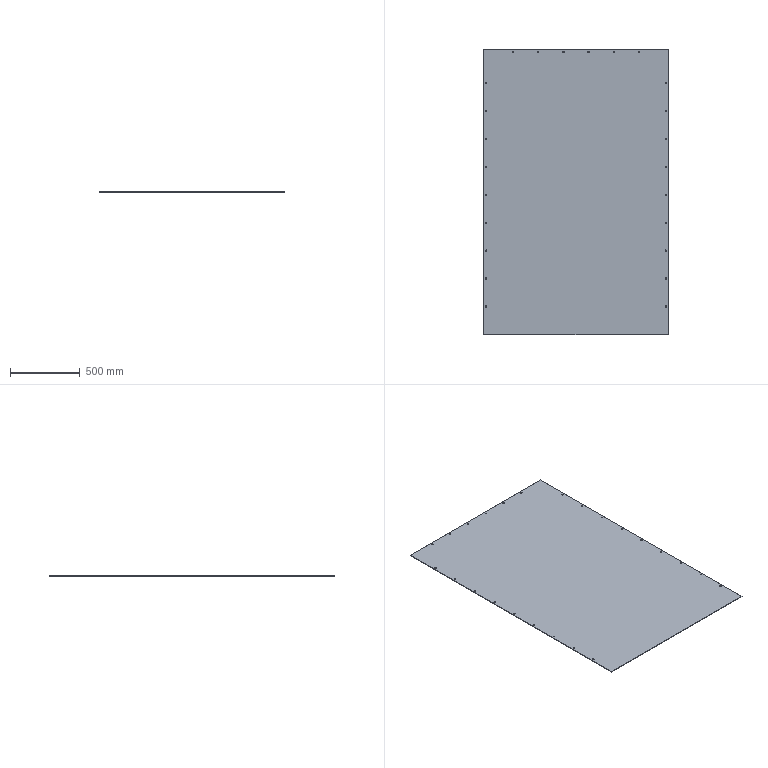Part | SolidWorks | features FlatPattern 1, SMBaseFlange 1, SheetMetal 1 | 1 solid | 54 faces | box 1320 x 2040 x 4 mm | volume 10763660 mm3 | cylinder 48 | plane 6 | commonest cylinder face diameters 10 x48